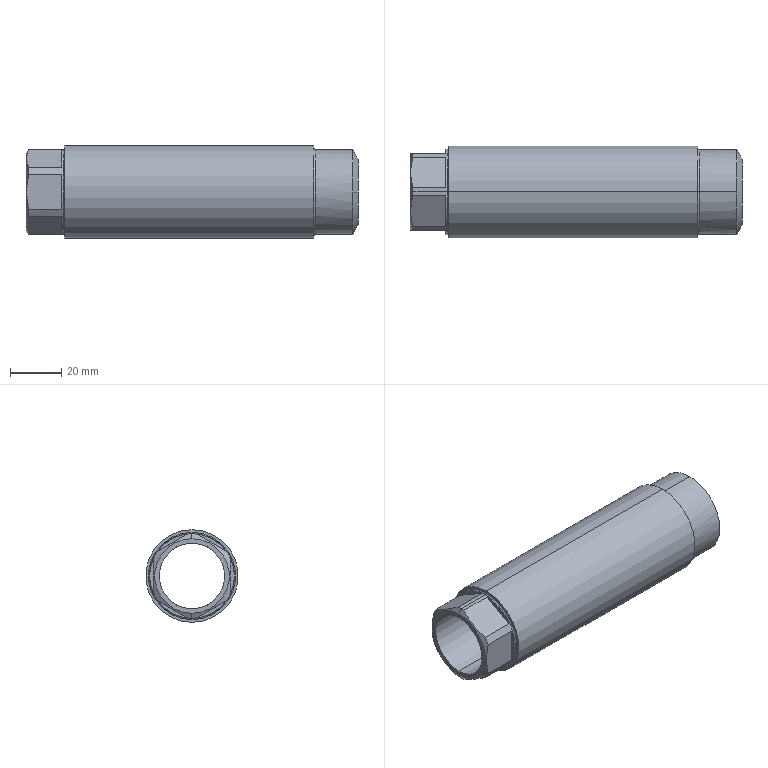Part | SolidWorks | features Cut 4, RevCut 2, Extrusion 1, Fillet 1 | 1 solid | 31 faces | box 129.156 x 36 x 36 mm | volume 58717 mm3 | plane 15 | cylinder 8 | torus 4 | cone 2 | sphere 2 | commonest cylinder face diameters 33 x4 25.5 x2 36 x2
STEP:
#1=CARTESIAN_POINT('',(0.,0.,-14.5));
#2=VERTEX_POINT('',#1);
#3=CARTESIAN_POINT('',(0.,0.,14.5));
#4=VERTEX_POINT('',#3);
#5=CARTESIAN_POINT('',(0.,0.,0.));
#6=DIRECTION('',(1.,0.,0.));
#7=DIRECTION('',(0.,0.,-1.));
#8=AXIS2_PLACEMENT_3D('',#5,#6,#7);
#9=CIRCLE('',#8,14.5);
#10=EDGE_CURVE('',#2,#4,#9,.T.);
#11=ORIENTED_EDGE('',*,*,#10,.T.);
#12=CARTESIAN_POINT('',(1.155,0.,16.5));
#13=VERTEX_POINT('',#12);
#14=CARTESIAN_POINT('',(5.774,0.,24.5));
#15=DIRECTION('',(0.5,0.,0.866));
#16=VECTOR('',#15,1000.);
#17=LINE('',#14,#16);
#18=EDGE_CURVE('',#4,#13,#17,.T.);
#19=ORIENTED_EDGE('',*,*,#18,.T.);
#20=CARTESIAN_POINT('',(1.155,1.547,16.427));
#21=VERTEX_POINT('',#20);
#22=CARTESIAN_POINT('',(1.155,0.,0.));
#23=DIRECTION('',(1.,0.,0.));
#24=DIRECTION('',(0.,0.,-1.));
#25=AXIS2_PLACEMENT_3D('',#22,#23,#24);
#26=CIRCLE('',#25,16.5);
#27=EDGE_CURVE('',#21,#13,#26,.T.);
#28=ORIENTED_EDGE('',*,*,#27,.F.);
#29=CARTESIAN_POINT('',(1.155,13.453,9.553));
#30=VERTEX_POINT('',#29);
#31=CARTESIAN_POINT('',(1.155,13.453,9.553));
#32=CARTESIAN_POINT('',(0.8829,12.474,10.119));
#33=CARTESIAN_POINT('',(0.6655,11.491,10.686));
#34=CARTESIAN_POINT('',(0.3687,9.515,11.827));
#35=CARTESIAN_POINT('',(0.2898,8.522,12.401));
#36=CARTESIAN_POINT('',(0.2881,7.022,13.266));
#37=CARTESIAN_POINT('',(0.3068,6.521,13.555));
#38=CARTESIAN_POINT('',(0.3828,5.516,14.136));
#39=CARTESIAN_POINT('',(0.44,5.013,14.426));
#40=CARTESIAN_POINT('',(0.6635,3.516,15.29));
#41=CARTESIAN_POINT('',(0.8823,2.528,15.861));
#42=CARTESIAN_POINT('',(1.155,1.547,16.427));
#43=B_SPLINE_CURVE_WITH_KNOTS('',3,(#31,#32,#33,#34,#35,#36,#37,#38,#39,#40,#41,#42),.UNSPECIFIED.,.F.,.F.,(4,2,2,2,2,4),(0.000000235,0.003449,0.006898,0.008623,0.01035,0.0138),.UNSPECIFIED.);
#44=EDGE_CURVE('',#30,#21,#43,.T.);
#45=ORIENTED_EDGE('',*,*,#44,.F.);
#46=CARTESIAN_POINT('',(1.155,15.,6.874));
#47=VERTEX_POINT('',#46);
#48=CARTESIAN_POINT('',(1.155,0.,0.));
#49=DIRECTION('',(1.,0.,0.));
#50=DIRECTION('',(0.,0.,-1.));
#51=AXIS2_PLACEMENT_3D('',#48,#49,#50);
#52=CIRCLE('',#51,16.5);
#53=EDGE_CURVE('',#47,#30,#52,.T.);
#54=ORIENTED_EDGE('',*,*,#53,.F.);
#55=CARTESIAN_POINT('',(1.155,15.,-6.874));
#56=VERTEX_POINT('',#55);
#57=CARTESIAN_POINT('',(1.155,15.,-6.874));
#58=CARTESIAN_POINT('',(0.8839,15.,-5.748));
#59=CARTESIAN_POINT('',(0.6635,15.,-4.599));
#60=CARTESIAN_POINT('',(0.3665,15.,-2.305));
#61=CARTESIAN_POINT('',(0.2888,15.,-1.155));
#62=CARTESIAN_POINT('',(0.2886,15.,1.15));
#63=CARTESIAN_POINT('',(0.3663,15.,2.307));
#64=CARTESIAN_POINT('',(0.6666,15.,4.619));
#65=CARTESIAN_POINT('',(0.8853,15.,5.754));
#66=CARTESIAN_POINT('',(1.155,15.,6.874));
#67=B_SPLINE_CURVE_WITH_KNOTS('',3,(#57,#58,#59,#60,#61,#62,#63,#64,#65,#66),.UNSPECIFIED.,.F.,.F.,(4,2,2,2,4),(0.01441,0.01786,0.02132,0.02477,0.02822),.UNSPECIFIED.);
#68=EDGE_CURVE('',#56,#47,#67,.T.);
#69=ORIENTED_EDGE('',*,*,#68,.F.);
#70=CARTESIAN_POINT('',(1.155,13.453,-9.553));
#71=VERTEX_POINT('',#70);
#72=CARTESIAN_POINT('',(1.155,0.,0.));
#73=DIRECTION('',(1.,0.,0.));
#74=DIRECTION('',(0.,0.,-1.));
#75=AXIS2_PLACEMENT_3D('',#72,#73,#74);
#76=CIRCLE('',#75,16.5);
#77=EDGE_CURVE('',#71,#56,#76,.T.);
#78=ORIENTED_EDGE('',*,*,#77,.F.);
#79=CARTESIAN_POINT('',(1.155,1.547,-16.427));
#80=VERTEX_POINT('',#79);
#81=CARTESIAN_POINT('',(1.155,1.547,-16.427));
#82=CARTESIAN_POINT('',(0.8829,2.526,-15.862));
#83=CARTESIAN_POINT('',(0.6655,3.509,-15.295));
#84=CARTESIAN_POINT('',(0.3687,5.485,-14.154));
#85=CARTESIAN_POINT('',(0.2898,6.478,-13.58));
#86=CARTESIAN_POINT('',(0.2881,7.978,-12.715));
#87=CARTESIAN_POINT('',(0.3068,8.479,-12.425));
#88=CARTESIAN_POINT('',(0.3828,9.484,-11.845));
#89=CARTESIAN_POINT('',(0.44,9.987,-11.555));
#90=CARTESIAN_POINT('',(0.6635,11.484,-10.69));
#91=CARTESIAN_POINT('',(0.8823,12.472,-10.12));
#92=CARTESIAN_POINT('',(1.155,13.453,-9.553));
#93=B_SPLINE_CURVE_WITH_KNOTS('',3,(#81,#82,#83,#84,#85,#86,#87,#88,#89,#90,#91,#92),.UNSPECIFIED.,.F.,.F.,(4,2,2,2,2,4),(0.000000235,0.003449,0.006898,0.008623,0.01035,0.0138),.UNSPECIFIED.);
#94=EDGE_CURVE('',#80,#71,#93,.T.);
#95=ORIENTED_EDGE('',*,*,#94,.F.);
#96=CARTESIAN_POINT('',(1.155,0.,-16.5));
#97=VERTEX_POINT('',#96);
#98=CARTESIAN_POINT('',(1.155,0.,0.));
#99=DIRECTION('',(1.,0.,0.));
#100=DIRECTION('',(0.,0.,-1.));
#101=AXIS2_PLACEMENT_3D('',#98,#99,#100);
#102=CIRCLE('',#101,16.5);
#103=EDGE_CURVE('',#97,#80,#102,.T.);
#104=ORIENTED_EDGE('',*,*,#103,.F.);
#105=CARTESIAN_POINT('',(5.774,0.,-24.5));
#106=DIRECTION('',(0.5,0.,-0.866));
#107=VECTOR('',#106,1000.);
#108=LINE('',#105,#107);
#109=EDGE_CURVE('',#2,#97,#108,.T.);
#110=ORIENTED_EDGE('',*,*,#109,.F.);
#111=EDGE_LOOP('',(#11,#19,#28,#45,#54,#69,#78,#95,#104,#110));
#112=FACE_OUTER_BOUND('',#111,.T.);
#113=CARTESIAN_POINT('',(5.774,0.,0.));
#114=DIRECTION('',(1.,0.,0.));
#115=DIRECTION('',(0.,0.,-1.));
#116=AXIS2_PLACEMENT_3D('',#113,#114,#115);
#117=CONICAL_SURFACE('',#116,24.5,1.047);
#118=ADVANCED_FACE('',(#112),#117,.T.);
#119=CARTESIAN_POINT('',(127.055,-16.5,0.));
#120=VERTEX_POINT('',#119);
#121=CARTESIAN_POINT('',(127.055,0.,16.5));
#122=VERTEX_POINT('',#121);
#123=CARTESIAN_POINT('',(127.055,0.,0.));
#124=DIRECTION('',(-1.,0.,0.));
#125=DIRECTION('',(0.,0.,1.));
#126=AXIS2_PLACEMENT_3D('',#123,#124,#125);
#127=CIRCLE('',#126,16.5);
#128=EDGE_CURVE('',#120,#122,#127,.T.);
#129=ORIENTED_EDGE('',*,*,#128,.F.);
#130=CARTESIAN_POINT('',(129.156,-12.75,0.));
#131=VERTEX_POINT('',#130);
#132=CARTESIAN_POINT('',(102.,0.,0.));
#133=DIRECTION('',(0.,0.,1.));
#134=DIRECTION('',(0.,-1.,0.));
#135=AXIS2_PLACEMENT_3D('',#132,#133,#134);
#136=CIRCLE('',#135,30.);
#137=EDGE_CURVE('',#120,#131,#136,.T.);
#138=ORIENTED_EDGE('',*,*,#137,.T.);
#139=CARTESIAN_POINT('',(129.156,0.,12.75));
#140=VERTEX_POINT('',#139);
#141=CARTESIAN_POINT('',(129.156,0.,0.));
#142=DIRECTION('',(-1.,0.,0.));
#143=DIRECTION('',(0.,0.,1.));
#144=AXIS2_PLACEMENT_3D('',#141,#142,#143);
#145=CIRCLE('',#144,12.75);
#146=EDGE_CURVE('',#131,#140,#145,.T.);
#147=ORIENTED_EDGE('',*,*,#146,.T.);
#148=CARTESIAN_POINT('',(129.156,12.75,0.));
#149=VERTEX_POINT('',#148);
#150=CARTESIAN_POINT('',(129.156,0.,0.));
#151=DIRECTION('',(-1.,0.,0.));
#152=DIRECTION('',(0.,0.,1.));
#153=AXIS2_PLACEMENT_3D('',#150,#151,#152);
#154=CIRCLE('',#153,12.75);
#155=EDGE_CURVE('',#140,#149,#154,.T.);
#156=ORIENTED_EDGE('',*,*,#155,.T.);
#157=CARTESIAN_POINT('',(127.055,16.5,0.));
#158=VERTEX_POINT('',#157);
#159=CARTESIAN_POINT('',(102.,0.,0.));
#160=DIRECTION('',(0.,0.,-1.));
#161=DIRECTION('',(-1.,0.,0.));
#162=AXIS2_PLACEMENT_3D('',#159,#160,#161);
#163=CIRCLE('',#162,30.);
#164=EDGE_CURVE('',#158,#149,#163,.T.);
#165=ORIENTED_EDGE('',*,*,#164,.F.);
#166=CARTESIAN_POINT('',(127.055,0.,0.));
#167=DIRECTION('',(-1.,0.,0.));
#168=DIRECTION('',(0.,0.,1.));
#169=AXIS2_PLACEMENT_3D('',#166,#167,#168);
#170=CIRCLE('',#169,16.5);
#171=EDGE_CURVE('',#122,#158,#170,.T.);
#172=ORIENTED_EDGE('',*,*,#171,.F.);
#173=EDGE_LOOP('',(#129,#138,#147,#156,#165,#172));
#174=FACE_OUTER_BOUND('',#173,.T.);
#175=CARTESIAN_POINT('',(102.,0.,0.));
#176=DIRECTION('',(0.,0.,1.));
#177=DIRECTION('',(0.,1.,0.));
#178=AXIS2_PLACEMENT_3D('',#175,#176,#177);
#179=SPHERICAL_SURFACE('',#178,30.);
#180=ADVANCED_FACE('',(#174),#179,.T.);
#181=CARTESIAN_POINT('',(112.5,0.,16.5));
#182=VERTEX_POINT('',#181);
#183=CARTESIAN_POINT('',(112.5,0.,-16.5));
#184=VERTEX_POINT('',#183);
#185=CARTESIAN_POINT('',(112.5,0.,0.));
#186=DIRECTION('',(1.,0.,0.));
#187=DIRECTION('',(0.,0.,-1.));
#188=AXIS2_PLACEMENT_3D('',#185,#186,#187);
#189=CIRCLE('',#188,16.5);
#190=EDGE_CURVE('',#182,#184,#189,.T.);
#191=ORIENTED_EDGE('',*,*,#190,.F.);
#192=CARTESIAN_POINT('',(112.,0.,17.));
#193=VERTEX_POINT('',#192);
#194=CARTESIAN_POINT('',(112.5,0.,17.));
#195=DIRECTION('',(0.,1.,0.));
#196=DIRECTION('',(0.,0.,1.));
#197=AXIS2_PLACEMENT_3D('',#194,#195,#196);
#198=CIRCLE('',#197,0.5);
#199=EDGE_CURVE('',#182,#193,#198,.T.);
#200=ORIENTED_EDGE('',*,*,#199,.T.);
#201=CARTESIAN_POINT('',(112.,0.,-17.));
#202=VERTEX_POINT('',#201);
#203=CARTESIAN_POINT('',(112.,0.,0.));
#204=DIRECTION('',(-1.,0.,0.));
#205=DIRECTION('',(0.,0.,-1.));
#206=AXIS2_PLACEMENT_3D('',#203,#204,#205);
#207=CIRCLE('',#206,17.);
#208=EDGE_CURVE('',#202,#193,#207,.T.);
#209=ORIENTED_EDGE('',*,*,#208,.F.);
#210=CARTESIAN_POINT('',(112.5,0.,-17.));
#211=DIRECTION('',(0.,-1.,0.));
#212=DIRECTION('',(0.,0.,-1.));
#213=AXIS2_PLACEMENT_3D('',#210,#211,#212);
#214=CIRCLE('',#213,0.5);
#215=EDGE_CURVE('',#184,#202,#214,.T.);
#216=ORIENTED_EDGE('',*,*,#215,.F.);
#217=EDGE_LOOP('',(#191,#200,#209,#216));
#218=FACE_OUTER_BOUND('',#217,.T.);
#219=CARTESIAN_POINT('',(112.5,0.,0.));
#220=DIRECTION('',(1.,0.,0.));
#221=DIRECTION('',(0.,0.,-1.));
#222=AXIS2_PLACEMENT_3D('',#219,#220,#221);
#223=TOROIDAL_SURFACE('',#222,17.,0.5);
#224=ADVANCED_FACE('',(#218),#223,.F.);
#225=CARTESIAN_POINT('',(14.5,0.,-16.5));
#226=VERTEX_POINT('',#225);
#227=CARTESIAN_POINT('',(14.5,0.,16.5));
#228=VERTEX_POINT('',#227);
#229=CARTESIAN_POINT('',(14.5,0.,0.));
#230=DIRECTION('',(-1.,0.,0.));
#231=DIRECTION('',(0.,0.,1.));
#232=AXIS2_PLACEMENT_3D('',#229,#230,#231);
#233=CIRCLE('',#232,16.5);
#234=EDGE_CURVE('',#226,#228,#233,.T.);
#235=ORIENTED_EDGE('',*,*,#234,.F.);
#236=CARTESIAN_POINT('',(15.,0.,-17.));
#237=VERTEX_POINT('',#236);
#238=CARTESIAN_POINT('',(14.5,0.,-17.));
#239=DIRECTION('',(0.,1.,0.));
#240=DIRECTION('',(0.,0.,1.));
#241=AXIS2_PLACEMENT_3D('',#238,#239,#240);
#242=CIRCLE('',#241,0.5);
#243=EDGE_CURVE('',#226,#237,#242,.T.);
#244=ORIENTED_EDGE('',*,*,#243,.T.);
#245=CARTESIAN_POINT('',(15.,0.,17.));
#246=VERTEX_POINT('',#245);
#247=CARTESIAN_POINT('',(15.,0.,0.));
#248=DIRECTION('',(1.,0.,0.));
#249=DIRECTION('',(0.,0.,1.));
#250=AXIS2_PLACEMENT_3D('',#247,#248,#249);
#251=CIRCLE('',#250,17.);
#252=EDGE_CURVE('',#246,#237,#251,.T.);
#253=ORIENTED_EDGE('',*,*,#252,.F.);
#254=CARTESIAN_POINT('',(14.5,0.,17.));
#255=DIRECTION('',(0.,-1.,0.));
#256=DIRECTION('',(0.,0.,-1.));
#257=AXIS2_PLACEMENT_3D('',#254,#255,#256);
#258=CIRCLE('',#257,0.5);
#259=EDGE_CURVE('',#228,#246,#258,.T.);
#260=ORIENTED_EDGE('',*,*,#259,.F.);
#261=EDGE_LOOP('',(#235,#244,#253,#260));
#262=FACE_OUTER_BOUND('',#261,.T.);
#263=CARTESIAN_POINT('',(14.5,0.,0.));
#264=DIRECTION('',(-1.,0.,0.));
#265=DIRECTION('',(0.,0.,1.));
#266=AXIS2_PLACEMENT_3D('',#263,#264,#265);
#267=TOROIDAL_SURFACE('',#266,17.,0.5);
#268=ADVANCED_FACE('',(#262),#267,.F.);
#269=CARTESIAN_POINT('',(112.,0.,-18.));
#270=VERTEX_POINT('',#269);
#271=CARTESIAN_POINT('',(112.,0.,18.));
#272=VERTEX_POINT('',#271);
#273=CARTESIAN_POINT('',(112.,0.,0.));
#274=DIRECTION('',(1.,0.,0.));
#275=DIRECTION('',(0.,0.,-1.));
#276=AXIS2_PLACEMENT_3D('',#273,#274,#275);
#277=CIRCLE('',#276,18.);
#278=EDGE_CURVE('',#270,#272,#277,.T.);
#279=ORIENTED_EDGE('',*,*,#278,.F.);
#280=CARTESIAN_POINT('',(15.,0.,-18.));
#281=VERTEX_POINT('',#280);
#282=CARTESIAN_POINT('',(132.,0.,-18.));
#283=DIRECTION('',(-1.,0.,0.));
#284=VECTOR('',#283,1000.);
#285=LINE('',#282,#284);
#286=EDGE_CURVE('',#270,#281,#285,.T.);
#287=ORIENTED_EDGE('',*,*,#286,.T.);
#288=CARTESIAN_POINT('',(15.,0.,18.));
#289=VERTEX_POINT('',#288);
#290=CARTESIAN_POINT('',(15.,0.,0.));
#291=DIRECTION('',(-1.,0.,0.));
#292=DIRECTION('',(0.,0.,1.));
#293=AXIS2_PLACEMENT_3D('',#290,#291,#292);
#294=CIRCLE('',#293,18.);
#295=EDGE_CURVE('',#289,#281,#294,.T.);
#296=ORIENTED_EDGE('',*,*,#295,.F.);
#297=CARTESIAN_POINT('',(132.,0.,18.));
#298=DIRECTION('',(-1.,0.,0.));
#299=VECTOR('',#298,1000.);
#300=LINE('',#297,#299);
#301=EDGE_CURVE('',#272,#289,#300,.T.);
#302=ORIENTED_EDGE('',*,*,#301,.F.);
#303=EDGE_LOOP('',(#279,#287,#296,#302));
#304=FACE_OUTER_BOUND('',#303,.T.);
#305=CARTESIAN_POINT('',(132.,0.,0.));
#306=DIRECTION('',(-1.,0.,0.));
#307=DIRECTION('',(0.,0.,1.));
#308=AXIS2_PLACEMENT_3D('',#305,#306,#307);
#309=CYLINDRICAL_SURFACE('',#308,18.);
#310=ADVANCED_FACE('',(#304),#309,.T.);
#311=CARTESIAN_POINT('',(112.5,0.,0.));
#312=DIRECTION('',(1.,0.,0.));
#313=DIRECTION('',(0.,0.,-1.));
#314=AXIS2_PLACEMENT_3D('',#311,#312,#313);
#315=CIRCLE('',#314,16.5);
#316=EDGE_CURVE('',#184,#182,#315,.T.);
#317=ORIENTED_EDGE('',*,*,#316,.T.);
#318=CARTESIAN_POINT('',(112.,0.,16.5));
#319=DIRECTION('',(1.,0.,0.));
#320=VECTOR('',#319,1000.);
#321=LINE('',#318,#320);
#322=EDGE_CURVE('',#182,#122,#321,.T.);
#323=ORIENTED_EDGE('',*,*,#322,.T.);
#324=ORIENTED_EDGE('',*,*,#171,.T.);
#325=CARTESIAN_POINT('',(127.055,0.,-16.5));
#326=VERTEX_POINT('',#325);
#327=CARTESIAN_POINT('',(127.055,0.,0.));
#328=DIRECTION('',(-1.,0.,0.));
#329=DIRECTION('',(0.,0.,1.));
#330=AXIS2_PLACEMENT_3D('',#327,#328,#329);
#331=CIRCLE('',#330,16.5);
#332=EDGE_CURVE('',#158,#326,#331,.T.);
#333=ORIENTED_EDGE('',*,*,#332,.T.);
#334=CARTESIAN_POINT('',(112.,0.,-16.5));
#335=DIRECTION('',(1.,0.,0.));
#336=VECTOR('',#335,1000.);
#337=LINE('',#334,#336);
#338=EDGE_CURVE('',#184,#326,#337,.T.);
#339=ORIENTED_EDGE('',*,*,#338,.F.);
#340=EDGE_LOOP('',(#317,#323,#324,#333,#339));
#341=FACE_OUTER_BOUND('',#340,.T.);
#342=CARTESIAN_POINT('',(112.,0.,0.));
#343=DIRECTION('',(1.,0.,0.));
#344=DIRECTION('',(0.,0.,-1.));
#345=AXIS2_PLACEMENT_3D('',#342,#343,#344);
#346=CYLINDRICAL_SURFACE('',#345,16.5);
#347=ADVANCED_FACE('',(#341),#346,.T.);
#348=CARTESIAN_POINT('',(129.156,0.,-12.75));
#349=VERTEX_POINT('',#348);
#350=CARTESIAN_POINT('',(129.156,0.,0.));
#351=DIRECTION('',(-1.,0.,0.));
#352=DIRECTION('',(0.,0.,1.));
#353=AXIS2_PLACEMENT_3D('',#350,#351,#352);
#354=CIRCLE('',#353,12.75);
#355=EDGE_CURVE('',#349,#131,#354,.T.);
#356=ORIENTED_EDGE('',*,*,#355,.F.);
#357=CARTESIAN_POINT('',(0.,0.,-12.75));
#358=VERTEX_POINT('',#357);
#359=CARTESIAN_POINT('',(132.,0.,-12.75));
#360=DIRECTION('',(-1.,0.,0.));
#361=VECTOR('',#360,1000.);
#362=LINE('',#359,#361);
#363=EDGE_CURVE('',#349,#358,#362,.T.);
#364=ORIENTED_EDGE('',*,*,#363,.T.);
#365=CARTESIAN_POINT('',(0.,0.,12.75));
#366=VERTEX_POINT('',#365);
#367=CARTESIAN_POINT('',(0.,0.,0.));
#368=DIRECTION('',(-1.,0.,0.));
#369=DIRECTION('',(0.,0.,1.));
#370=AXIS2_PLACEMENT_3D('',#367,#368,#369);
#371=CIRCLE('',#370,12.75);
#372=EDGE_CURVE('',#358,#366,#371,.T.);
#373=ORIENTED_EDGE('',*,*,#372,.T.);
#374=CARTESIAN_POINT('',(132.,0.,12.75));
#375=DIRECTION('',(-1.,0.,0.));
#376=VECTOR('',#375,1000.);
#377=LINE('',#374,#376);
#378=EDGE_CURVE('',#140,#366,#377,.T.);
#379=ORIENTED_EDGE('',*,*,#378,.F.);
#380=ORIENTED_EDGE('',*,*,#146,.F.);
#381=EDGE_LOOP('',(#356,#364,#373,#379,#380));
#382=FACE_OUTER_BOUND('',#381,.T.);
#383=CARTESIAN_POINT('',(132.,0.,0.));
#384=DIRECTION('',(-1.,0.,0.));
#385=DIRECTION('',(0.,0.,1.));
#386=AXIS2_PLACEMENT_3D('',#383,#384,#385);
#387=CYLINDRICAL_SURFACE('',#386,12.75);
#388=ADVANCED_FACE('',(#382),#387,.F.);
#389=CARTESIAN_POINT('',(14.5,0.,0.));
#390=DIRECTION('',(-1.,0.,0.));
#391=DIRECTION('',(0.,0.,1.));
#392=AXIS2_PLACEMENT_3D('',#389,#390,#391);
#393=CIRCLE('',#392,16.5);
#394=EDGE_CURVE('',#228,#226,#393,.T.);
#395=ORIENTED_EDGE('',*,*,#394,.T.);
#396=CARTESIAN_POINT('',(15.,0.,-16.5));
#397=DIRECTION('',(-1.,0.,0.));
#398=VECTOR('',#397,1000.);
#399=LINE('',#396,#398);
#400=EDGE_CURVE('',#226,#97,#399,.T.);
#401=ORIENTED_EDGE('',*,*,#400,.T.);
#402=ORIENTED_EDGE('',*,*,#103,.T.);
#403=CARTESIAN_POINT('',(14.,1.547,-16.427));
#404=VERTEX_POINT('',#403);
#405=CARTESIAN_POINT('',(15.,1.547,-16.427));
#406=DIRECTION('',(1.,0.,0.));
#407=VECTOR('',#406,1000.);
#408=LINE('',#405,#407);
#409=EDGE_CURVE('',#80,#404,#408,.T.);
#410=ORIENTED_EDGE('',*,*,#409,.T.);
#411=CARTESIAN_POINT('',(14.,13.453,-9.553));
#412=VERTEX_POINT('',#411);
#413=CARTESIAN_POINT('',(14.,0.,0.));
#414=DIRECTION('',(1.,0.,0.));
#415=DIRECTION('',(0.,0.,1.));
#416=AXIS2_PLACEMENT_3D('',#413,#414,#415);
#417=CIRCLE('',#416,16.5);
#418=EDGE_CURVE('',#404,#412,#417,.T.);
#419=ORIENTED_EDGE('',*,*,#418,.T.);
#420=CARTESIAN_POINT('',(15.,13.453,-9.553));
#421=DIRECTION('',(-1.,0.,0.));
#422=VECTOR('',#421,1000.);
#423=LINE('',#420,#422);
#424=EDGE_CURVE('',#412,#71,#423,.T.);
#425=ORIENTED_EDGE('',*,*,#424,.T.);
#426=ORIENTED_EDGE('',*,*,#77,.T.);
#427=CARTESIAN_POINT('',(14.,15.,-6.874));
#428=VERTEX_POINT('',#427);
#429=CARTESIAN_POINT('',(15.,15.,-6.874));
#430=DIRECTION('',(1.,0.,0.));
#431=VECTOR('',#430,1000.);
#432=LINE('',#429,#431);
#433=EDGE_CURVE('',#56,#428,#432,.T.);
#434=ORIENTED_EDGE('',*,*,#433,.T.);
#435=CARTESIAN_POINT('',(14.,15.,6.874));
#436=VERTEX_POINT('',#435);
#437=CARTESIAN_POINT('',(14.,0.,0.));
#438=DIRECTION('',(1.,0.,0.));
#439=DIRECTION('',(0.,0.,1.));
#440=AXIS2_PLACEMENT_3D('',#437,#438,#439);
#441=CIRCLE('',#440,16.5);
#442=EDGE_CURVE('',#428,#436,#441,.T.);
#443=ORIENTED_EDGE('',*,*,#442,.T.);
#444=CARTESIAN_POINT('',(15.,15.,6.874));
#445=DIRECTION('',(-1.,0.,0.));
#446=VECTOR('',#445,1000.);
#447=LINE('',#444,#446);
#448=EDGE_CURVE('',#436,#47,#447,.T.);
#449=ORIENTED_EDGE('',*,*,#448,.T.);
#450=ORIENTED_EDGE('',*,*,#53,.T.);
#451=CARTESIAN_POINT('',(14.,13.453,9.553));
#452=VERTEX_POINT('',#451);
#453=CARTESIAN_POINT('',(15.,13.453,9.553));
#454=DIRECTION('',(1.,0.,0.));
#455=VECTOR('',#454,1000.);
#456=LINE('',#453,#455);
#457=EDGE_CURVE('',#30,#452,#456,.T.);
#458=ORIENTED_EDGE('',*,*,#457,.T.);
#459=CARTESIAN_POINT('',(14.,1.547,16.427));
#460=VERTEX_POINT('',#459);
#461=CARTESIAN_POINT('',(14.,0.,0.));
#462=DIRECTION('',(1.,0.,0.));
#463=DIRECTION('',(0.,0.,1.));
#464=AXIS2_PLACEMENT_3D('',#461,#462,#463);
#465=CIRCLE('',#464,16.5);
#466=EDGE_CURVE('',#452,#460,#465,.T.);
#467=ORIENTED_EDGE('',*,*,#466,.T.);
#468=CARTESIAN_POINT('',(15.,1.547,16.427));
#469=DIRECTION('',(-1.,0.,0.));
#470=VECTOR('',#469,1000.);
#471=LINE('',#468,#470);
#472=EDGE_CURVE('',#460,#21,#471,.T.);
#473=ORIENTED_EDGE('',*,*,#472,.T.);
#474=ORIENTED_EDGE('',*,*,#27,.T.);
#475=CARTESIAN_POINT('',(15.,0.,16.5));
#476=DIRECTION('',(-1.,0.,0.));
#477=VECTOR('',#476,1000.);
#478=LINE('',#475,#477);
#479=EDGE_CURVE('',#228,#13,#478,.T.);
#480=ORIENTED_EDGE('',*,*,#479,.F.);
#481=EDGE_LOOP('',(#395,#401,#402,#410,#419,#425,#426,#434,#443,#449,#450,#458,#467,#473,#474,#480));
#482=FACE_OUTER_BOUND('',#481,.T.);
#483=CARTESIAN_POINT('',(15.,0.,0.));
#484=DIRECTION('',(-1.,0.,0.));
#485=DIRECTION('',(0.,0.,1.));
#486=AXIS2_PLACEMENT_3D('',#483,#484,#485);
#487=CYLINDRICAL_SURFACE('',#486,16.5);
#488=ADVANCED_FACE('',(#482),#487,.T.);
#489=CARTESIAN_POINT('',(0.,0.,0.));
#490=DIRECTION('',(-1.,0.,0.));
#491=DIRECTION('',(0.,0.,1.));
#492=AXIS2_PLACEMENT_3D('',#489,#490,#491);
#493=CIRCLE('',#492,12.75);
#494=EDGE_CURVE('',#366,#358,#493,.T.);
#495=ORIENTED_EDGE('',*,*,#494,.F.);
#496=ORIENTED_EDGE('',*,*,#372,.F.);
#497=EDGE_LOOP('',(#495,#496));
#498=FACE_BOUND('',#497,.T.);
#499=ORIENTED_EDGE('',*,*,#10,.F.);
#500=CARTESIAN_POINT('',(0.,0.,0.));
#501=DIRECTION('',(1.,0.,0.));
#502=DIRECTION('',(0.,0.,-1.));
#503=AXIS2_PLACEMENT_3D('',#500,#501,#502);
#504=CIRCLE('',#503,14.5);
#505=EDGE_CURVE('',#4,#2,#504,.T.);
#506=ORIENTED_EDGE('',*,*,#505,.F.);
#507=EDGE_LOOP('',(#499,#506));
#508=FACE_OUTER_BOUND('',#507,.T.);
#509=CARTESIAN_POINT('',(0.,0.,0.));
#510=DIRECTION('',(1.,0.,0.));
#511=DIRECTION('',(0.,0.,-1.));
#512=AXIS2_PLACEMENT_3D('',#509,#510,#511);
#513=PLANE('',#512);
#514=ADVANCED_FACE('',(#498,#508),#513,.F.);
#515=ORIENTED_EDGE('',*,*,#400,.F.);
#516=ORIENTED_EDGE('',*,*,#234,.T.);
#517=ORIENTED_EDGE('',*,*,#479,.T.);
#518=CARTESIAN_POINT('',(1.155,-1.547,16.427));
#519=VERTEX_POINT('',#518);
#520=CARTESIAN_POINT('',(1.155,0.,0.));
#521=DIRECTION('',(1.,0.,0.));
#522=DIRECTION('',(0.,0.,-1.));
#523=AXIS2_PLACEMENT_3D('',#520,#521,#522);
#524=CIRCLE('',#523,16.5);
#525=EDGE_CURVE('',#13,#519,#524,.T.);
#526=ORIENTED_EDGE('',*,*,#525,.T.);
#527=CARTESIAN_POINT('',(14.,-1.547,16.427));
#528=VERTEX_POINT('',#527);
#529=CARTESIAN_POINT('',(15.,-1.547,16.427));
#530=DIRECTION('',(1.,0.,0.));
#531=VECTOR('',#530,1000.);
#532=LINE('',#529,#531);
#533=EDGE_CURVE('',#519,#528,#532,.T.);
#534=ORIENTED_EDGE('',*,*,#533,.T.);
#535=CARTESIAN_POINT('',(14.,-13.453,9.553));
#536=VERTEX_POINT('',#535);
#537=CARTESIAN_POINT('',(14.,0.,0.));
#538=DIRECTION('',(1.,0.,0.));
#539=DIRECTION('',(0.,0.,1.));
#540=AXIS2_PLACEMENT_3D('',#537,#538,#539);
#541=CIRCLE('',#540,16.5);
#542=EDGE_CURVE('',#528,#536,#541,.T.);
#543=ORIENTED_EDGE('',*,*,#542,.T.);
#544=CARTESIAN_POINT('',(1.155,-13.453,9.553));
#545=VERTEX_POINT('',#544);
#546=CARTESIAN_POINT('',(15.,-13.453,9.553));
#547=DIRECTION('',(-1.,0.,0.));
#548=VECTOR('',#547,1000.);
#549=LINE('',#546,#548);
#550=EDGE_CURVE('',#536,#545,#549,.T.);
#551=ORIENTED_EDGE('',*,*,#550,.T.);
#552=CARTESIAN_POINT('',(1.155,-15.,6.874));
#553=VERTEX_POINT('',#552);
#554=CARTESIAN_POINT('',(1.155,0.,0.));
#555=DIRECTION('',(1.,0.,0.));
#556=DIRECTION('',(0.,0.,-1.));
#557=AXIS2_PLACEMENT_3D('',#554,#555,#556);
#558=CIRCLE('',#557,16.5);
#559=EDGE_CURVE('',#545,#553,#558,.T.);
#560=ORIENTED_EDGE('',*,*,#559,.T.);
#561=CARTESIAN_POINT('',(14.,-15.,6.874));
#562=VERTEX_POINT('',#561);
#563=CARTESIAN_POINT('',(15.,-15.,6.874));
#564=DIRECTION('',(1.,0.,0.));
#565=VECTOR('',#564,1000.);
#566=LINE('',#563,#565);
#567=EDGE_CURVE('',#553,#562,#566,.T.);
#568=ORIENTED_EDGE('',*,*,#567,.T.);
#569=CARTESIAN_POINT('',(14.,-15.,-6.874));
#570=VERTEX_POINT('',#569);
#571=CARTESIAN_POINT('',(14.,0.,0.));
#572=DIRECTION('',(1.,0.,0.));
#573=DIRECTION('',(0.,0.,1.));
#574=AXIS2_PLACEMENT_3D('',#571,#572,#573);
#575=CIRCLE('',#574,16.5);
#576=EDGE_CURVE('',#562,#570,#575,.T.);
#577=ORIENTED_EDGE('',*,*,#576,.T.);
#578=CARTESIAN_POINT('',(1.155,-15.,-6.874));
#579=VERTEX_POINT('',#578);
#580=CARTESIAN_POINT('',(15.,-15.,-6.874));
#581=DIRECTION('',(-1.,0.,0.));
#582=VECTOR('',#581,1000.);
#583=LINE('',#580,#582);
#584=EDGE_CURVE('',#570,#579,#583,.T.);
#585=ORIENTED_EDGE('',*,*,#584,.T.);
#586=CARTESIAN_POINT('',(1.155,-13.453,-9.553));
#587=VERTEX_POINT('',#586);
#588=CARTESIAN_POINT('',(1.155,0.,0.));
#589=DIRECTION('',(1.,0.,0.));
#590=DIRECTION('',(0.,0.,-1.));
#591=AXIS2_PLACEMENT_3D('',#588,#589,#590);
#592=CIRCLE('',#591,16.5);
#593=EDGE_CURVE('',#579,#587,#592,.T.);
#594=ORIENTED_EDGE('',*,*,#593,.T.);
#595=CARTESIAN_POINT('',(14.,-13.453,-9.553));
#596=VERTEX_POINT('',#595);
#597=CARTESIAN_POINT('',(15.,-13.453,-9.553));
#598=DIRECTION('',(1.,0.,0.));
#599=VECTOR('',#598,1000.);
#600=LINE('',#597,#599);
#601=EDGE_CURVE('',#587,#596,#600,.T.);
#602=ORIENTED_EDGE('',*,*,#601,.T.);
#603=CARTESIAN_POINT('',(14.,-1.547,-16.427));
#604=VERTEX_POINT('',#603);
#605=CARTESIAN_POINT('',(14.,0.,0.));
#606=DIRECTION('',(1.,0.,0.));
#607=DIRECTION('',(0.,0.,1.));
#608=AXIS2_PLACEMENT_3D('',#605,#606,#607);
#609=CIRCLE('',#608,16.5);
#610=EDGE_CURVE('',#596,#604,#609,.T.);
#611=ORIENTED_EDGE('',*,*,#610,.T.);
#612=CARTESIAN_POINT('',(1.155,-1.547,-16.427));
#613=VERTEX_POINT('',#612);
#614=CARTESIAN_POINT('',(15.,-1.547,-16.427));
#615=DIRECTION('',(-1.,0.,0.));
#616=VECTOR('',#615,1000.);
#617=LINE('',#614,#616);
#618=EDGE_CURVE('',#604,#613,#617,.T.);
#619=ORIENTED_EDGE('',*,*,#618,.T.);
#620=CARTESIAN_POINT('',(1.155,0.,0.));
#621=DIRECTION('',(1.,0.,0.));
#622=DIRECTION('',(0.,0.,-1.));
#623=AXIS2_PLACEMENT_3D('',#620,#621,#622);
#624=CIRCLE('',#623,16.5);
#625=EDGE_CURVE('',#613,#97,#624,.T.);
#626=ORIENTED_EDGE('',*,*,#625,.T.);
#627=EDGE_LOOP('',(#515,#516,#517,#526,#534,#543,#551,#560,#568,#577,#585,#594,#602,#611,#619,#626));
#628=FACE_OUTER_BOUND('',#627,.T.);
#629=CARTESIAN_POINT('',(15.,0.,0.));
#630=DIRECTION('',(-1.,0.,0.));
#631=DIRECTION('',(0.,0.,1.));
#632=AXIS2_PLACEMENT_3D('',#629,#630,#631);
#633=CYLINDRICAL_SURFACE('',#632,16.5);
#634=ADVANCED_FACE('',(#628),#633,.T.);
#635=ORIENTED_EDGE('',*,*,#567,.F.);
#636=CARTESIAN_POINT('',(1.155,-15.,6.874));
#637=CARTESIAN_POINT('',(0.8853,-15.,5.754));
#638=CARTESIAN_POINT('',(0.6666,-15.,4.619));
#639=CARTESIAN_POINT('',(0.3663,-15.,2.307));
#640=CARTESIAN_POINT('',(0.2886,-15.,1.15));
#641=CARTESIAN_POINT('',(0.2888,-15.,-1.155));
#642=CARTESIAN_POINT('',(0.3665,-15.,-2.305));
#643=CARTESIAN_POINT('',(0.6635,-15.,-4.599));
#644=CARTESIAN_POINT('',(0.8839,-15.,-5.748));
#645=CARTESIAN_POINT('',(1.155,-15.,-6.874));
#646=B_SPLINE_CURVE_WITH_KNOTS('',3,(#636,#637,#638,#639,#640,#641,#642,#643,#644,#645),.UNSPECIFIED.,.F.,.F.,(4,2,2,2,4),(0.01016,0.01361,0.01705,0.0205,0.02395),.UNSPECIFIED.);
#647=EDGE_CURVE('',#553,#579,#646,.T.);
#648=ORIENTED_EDGE('',*,*,#647,.T.);
#649=ORIENTED_EDGE('',*,*,#584,.F.);
#650=CARTESIAN_POINT('',(14.,-15.,-8.66));
#651=DIRECTION('',(0.,0.,1.));
#652=VECTOR('',#651,1000.);
#653=LINE('',#650,#652);
#654=EDGE_CURVE('',#570,#562,#653,.T.);
#655=ORIENTED_EDGE('',*,*,#654,.T.);
#656=EDGE_LOOP('',(#635,#648,#649,#655));
#657=FACE_OUTER_BOUND('',#656,.T.);
#658=CARTESIAN_POINT('',(14.,-15.,-8.66));
#659=DIRECTION('',(0.,-1.,0.));
#660=DIRECTION('',(0.,0.,-1.));
#661=AXIS2_PLACEMENT_3D('',#658,#659,#660);
#662=PLANE('',#661);
#663=ADVANCED_FACE('',(#657),#662,.T.);
#664=ORIENTED_EDGE('',*,*,#533,.F.);
#665=CARTESIAN_POINT('',(1.155,-1.547,16.427));
#666=CARTESIAN_POINT('',(0.8829,-2.526,15.862));
#667=CARTESIAN_POINT('',(0.6655,-3.509,15.295));
#668=CARTESIAN_POINT('',(0.3687,-5.485,14.154));
#669=CARTESIAN_POINT('',(0.2898,-6.478,13.58));
#670=CARTESIAN_POINT('',(0.2881,-7.978,12.715));
#671=CARTESIAN_POINT('',(0.3068,-8.479,12.425));
#672=CARTESIAN_POINT('',(0.3828,-9.484,11.845));
#673=CARTESIAN_POINT('',(0.44,-9.987,11.555));
#674=CARTESIAN_POINT('',(0.6635,-11.484,10.69));
#675=CARTESIAN_POINT('',(0.8823,-12.472,10.12));
#676=CARTESIAN_POINT('',(1.155,-13.453,9.553));
#677=B_SPLINE_CURVE_WITH_KNOTS('',3,(#665,#666,#667,#668,#669,#670,#671,#672,#673,#674,#675,#676),.UNSPECIFIED.,.F.,.F.,(4,2,2,2,2,4),(0.000000235,0.003449,0.006898,0.008623,0.01035,0.0138),.UNSPECIFIED.);
#678=EDGE_CURVE('',#519,#545,#677,.T.);
#679=ORIENTED_EDGE('',*,*,#678,.T.);
#680=ORIENTED_EDGE('',*,*,#550,.F.);
#681=CARTESIAN_POINT('',(14.,-15.,8.66));
#682=DIRECTION('',(0.,0.866,0.5));
#683=VECTOR('',#682,1000.);
#684=LINE('',#681,#683);
#685=EDGE_CURVE('',#536,#528,#684,.T.);
#686=ORIENTED_EDGE('',*,*,#685,.T.);
#687=EDGE_LOOP('',(#664,#679,#680,#686));
#688=FACE_OUTER_BOUND('',#687,.T.);
#689=CARTESIAN_POINT('',(14.,-15.,8.66));
#690=DIRECTION('',(0.,-0.5,0.866));
#691=DIRECTION('',(0.,-0.866,-0.5));
#692=AXIS2_PLACEMENT_3D('',#689,#690,#691);
#693=PLANE('',#692);
#694=ADVANCED_FACE('',(#688),#693,.T.);
#695=ORIENTED_EDGE('',*,*,#457,.F.);
#696=ORIENTED_EDGE('',*,*,#44,.T.);
#697=ORIENTED_EDGE('',*,*,#472,.F.);
#698=CARTESIAN_POINT('',(14.,0.,17.321));
#699=DIRECTION('',(0.,0.866,-0.5));
#700=VECTOR('',#699,1000.);
#701=LINE('',#698,#700);
#702=EDGE_CURVE('',#460,#452,#701,.T.);
#703=ORIENTED_EDGE('',*,*,#702,.T.);
#704=EDGE_LOOP('',(#695,#696,#697,#703));
#705=FACE_OUTER_BOUND('',#704,.T.);
#706=CARTESIAN_POINT('',(14.,0.,17.321));
#707=DIRECTION('',(0.,0.5,0.866));
#708=DIRECTION('',(0.,-0.866,0.5));
#709=AXIS2_PLACEMENT_3D('',#706,#707,#708);
#710=PLANE('',#709);
#711=ADVANCED_FACE('',(#705),#710,.T.);
#712=ORIENTED_EDGE('',*,*,#433,.F.);
#713=ORIENTED_EDGE('',*,*,#68,.T.);
#714=ORIENTED_EDGE('',*,*,#448,.F.);
#715=CARTESIAN_POINT('',(14.,15.,8.66));
#716=DIRECTION('',(0.,0.,-1.));
#717=VECTOR('',#716,1000.);
#718=LINE('',#715,#717);
#719=EDGE_CURVE('',#436,#428,#718,.T.);
#720=ORIENTED_EDGE('',*,*,#719,.T.);
#721=EDGE_LOOP('',(#712,#713,#714,#720));
#722=FACE_OUTER_BOUND('',#721,.T.);
#723=CARTESIAN_POINT('',(14.,15.,8.66));
#724=DIRECTION('',(0.,1.,0.));
#725=DIRECTION('',(0.,0.,1.));
#726=AXIS2_PLACEMENT_3D('',#723,#724,#725);
#727=PLANE('',#726);
#728=ADVANCED_FACE('',(#722),#727,.T.);
#729=ORIENTED_EDGE('',*,*,#409,.F.);
#730=ORIENTED_EDGE('',*,*,#94,.T.);
#731=ORIENTED_EDGE('',*,*,#424,.F.);
#732=CARTESIAN_POINT('',(14.,15.,-8.66));
#733=DIRECTION('',(0.,-0.866,-0.5));
#734=VECTOR('',#733,1000.);
#735=LINE('',#732,#734);
#736=EDGE_CURVE('',#412,#404,#735,.T.);
#737=ORIENTED_EDGE('',*,*,#736,.T.);
#738=EDGE_LOOP('',(#729,#730,#731,#737));
#739=FACE_OUTER_BOUND('',#738,.T.);
#740=CARTESIAN_POINT('',(14.,15.,-8.66));
#741=DIRECTION('',(0.,0.5,-0.866));
#742=DIRECTION('',(0.,0.866,0.5));
#743=AXIS2_PLACEMENT_3D('',#740,#741,#742);
#744=PLANE('',#743);
#745=ADVANCED_FACE('',(#739),#744,.T.);
#746=ORIENTED_EDGE('',*,*,#601,.F.);
#747=CARTESIAN_POINT('',(1.155,-13.453,-9.553));
#748=CARTESIAN_POINT('',(0.8829,-12.474,-10.119));
#749=CARTESIAN_POINT('',(0.6655,-11.491,-10.686));
#750=CARTESIAN_POINT('',(0.3687,-9.515,-11.827));
#751=CARTESIAN_POINT('',(0.2898,-8.522,-12.401));
#752=CARTESIAN_POINT('',(0.2881,-7.022,-13.266));
#753=CARTESIAN_POINT('',(0.3068,-6.521,-13.555));
#754=CARTESIAN_POINT('',(0.3828,-5.516,-14.136));
#755=CARTESIAN_POINT('',(0.44,-5.013,-14.426));
#756=CARTESIAN_POINT('',(0.6635,-3.516,-15.29));
#757=CARTESIAN_POINT('',(0.8823,-2.528,-15.861));
#758=CARTESIAN_POINT('',(1.155,-1.547,-16.427));
#759=B_SPLINE_CURVE_WITH_KNOTS('',3,(#747,#748,#749,#750,#751,#752,#753,#754,#755,#756,#757,#758),.UNSPECIFIED.,.F.,.F.,(4,2,2,2,2,4),(0.000000235,0.003449,0.006898,0.008623,0.01035,0.0138),.UNSPECIFIED.);
#760=EDGE_CURVE('',#587,#613,#759,.T.);
#761=ORIENTED_EDGE('',*,*,#760,.T.);
#762=ORIENTED_EDGE('',*,*,#618,.F.);
#763=CARTESIAN_POINT('',(14.,0.,-17.321));
#764=DIRECTION('',(0.,-0.866,0.5));
#765=VECTOR('',#764,1000.);
#766=LINE('',#763,#765);
#767=EDGE_CURVE('',#604,#596,#766,.T.);
#768=ORIENTED_EDGE('',*,*,#767,.T.);
#769=EDGE_LOOP('',(#746,#761,#762,#768));
#770=FACE_OUTER_BOUND('',#769,.T.);
#771=CARTESIAN_POINT('',(14.,0.,-17.321));
#772=DIRECTION('',(0.,-0.5,-0.866));
#773=DIRECTION('',(0.,0.866,-0.5));
#774=AXIS2_PLACEMENT_3D('',#771,#772,#773);
#775=PLANE('',#774);
#776=ADVANCED_FACE('',(#770),#775,.T.);
#777=ORIENTED_EDGE('',*,*,#363,.F.);
#778=CARTESIAN_POINT('',(129.156,0.,0.));
#779=DIRECTION('',(-1.,0.,0.));
#780=DIRECTION('',(0.,0.,1.));
#781=AXIS2_PLACEMENT_3D('',#778,#779,#780);
#782=CIRCLE('',#781,12.75);
#783=EDGE_CURVE('',#149,#349,#782,.T.);
#784=ORIENTED_EDGE('',*,*,#783,.F.);
#785=ORIENTED_EDGE('',*,*,#155,.F.);
#786=ORIENTED_EDGE('',*,*,#378,.T.);
#787=ORIENTED_EDGE('',*,*,#494,.T.);
#788=EDGE_LOOP('',(#777,#784,#785,#786,#787));
#789=FACE_OUTER_BOUND('',#788,.T.);
#790=CARTESIAN_POINT('',(132.,0.,0.));
#791=DIRECTION('',(-1.,0.,0.));
#792=DIRECTION('',(0.,0.,1.));
#793=AXIS2_PLACEMENT_3D('',#790,#791,#792);
#794=CYLINDRICAL_SURFACE('',#793,12.75);
#795=ADVANCED_FACE('',(#789),#794,.F.);
#796=ORIENTED_EDGE('',*,*,#322,.F.);
#797=ORIENTED_EDGE('',*,*,#190,.T.);
#798=ORIENTED_EDGE('',*,*,#338,.T.);
#799=CARTESIAN_POINT('',(127.055,0.,0.));
#800=DIRECTION('',(-1.,0.,0.));
#801=DIRECTION('',(0.,0.,1.));
#802=AXIS2_PLACEMENT_3D('',#799,#800,#801);
#803=CIRCLE('',#802,16.5);
#804=EDGE_CURVE('',#326,#120,#803,.T.);
#805=ORIENTED_EDGE('',*,*,#804,.T.);
#806=ORIENTED_EDGE('',*,*,#128,.T.);
#807=EDGE_LOOP('',(#796,#797,#798,#805,#806));
#808=FACE_OUTER_BOUND('',#807,.T.);
#809=CARTESIAN_POINT('',(112.,0.,0.));
#810=DIRECTION('',(1.,0.,0.));
#811=DIRECTION('',(0.,0.,-1.));
#812=AXIS2_PLACEMENT_3D('',#809,#810,#811);
#813=CYLINDRICAL_SURFACE('',#812,16.5);
#814=ADVANCED_FACE('',(#808),#813,.T.);
#815=ORIENTED_EDGE('',*,*,#286,.F.);
#816=CARTESIAN_POINT('',(112.,0.,0.));
#817=DIRECTION('',(1.,0.,0.));
#818=DIRECTION('',(0.,0.,-1.));
#819=AXIS2_PLACEMENT_3D('',#816,#817,#818);
#820=CIRCLE('',#819,18.);
#821=EDGE_CURVE('',#272,#270,#820,.T.);
#822=ORIENTED_EDGE('',*,*,#821,.F.);
#823=ORIENTED_EDGE('',*,*,#301,.T.);
#824=CARTESIAN_POINT('',(15.,0.,0.));
#825=DIRECTION('',(-1.,0.,0.));
#826=DIRECTION('',(0.,0.,1.));
#827=AXIS2_PLACEMENT_3D('',#824,#825,#826);
#828=CIRCLE('',#827,18.);
#829=EDGE_CURVE('',#281,#289,#828,.T.);
#830=ORIENTED_EDGE('',*,*,#829,.F.);
#831=EDGE_LOOP('',(#815,#822,#823,#830));
#832=FACE_OUTER_BOUND('',#831,.T.);
#833=CARTESIAN_POINT('',(132.,0.,0.));
#834=DIRECTION('',(-1.,0.,0.));
#835=DIRECTION('',(0.,0.,1.));
#836=AXIS2_PLACEMENT_3D('',#833,#834,#835);
#837=CYLINDRICAL_SURFACE('',#836,18.);
#838=ADVANCED_FACE('',(#832),#837,.T.);
#839=ORIENTED_EDGE('',*,*,#252,.T.);
#840=CARTESIAN_POINT('',(15.,0.,0.));
#841=DIRECTION('',(1.,0.,0.));
#842=DIRECTION('',(0.,0.,1.));
#843=AXIS2_PLACEMENT_3D('',#840,#841,#842);
#844=CIRCLE('',#843,17.);
#845=EDGE_CURVE('',#237,#246,#844,.T.);
#846=ORIENTED_EDGE('',*,*,#845,.T.);
#847=EDGE_LOOP('',(#839,#846));
#848=FACE_BOUND('',#847,.T.);
#849=ORIENTED_EDGE('',*,*,#295,.T.);
#850=ORIENTED_EDGE('',*,*,#829,.T.);
#851=EDGE_LOOP('',(#849,#850));
#852=FACE_OUTER_BOUND('',#851,.T.);
#853=CARTESIAN_POINT('',(15.,0.,0.));
#854=DIRECTION('',(-1.,0.,0.));
#855=DIRECTION('',(0.,0.,1.));
#856=AXIS2_PLACEMENT_3D('',#853,#854,#855);
#857=PLANE('',#856);
#858=ADVANCED_FACE('',(#848,#852),#857,.T.);
#859=ORIENTED_EDGE('',*,*,#208,.T.);
#860=CARTESIAN_POINT('',(112.,0.,0.));
#861=DIRECTION('',(-1.,0.,0.));
#862=DIRECTION('',(0.,0.,-1.));
#863=AXIS2_PLACEMENT_3D('',#860,#861,#862);
#864=CIRCLE('',#863,17.);
#865=EDGE_CURVE('',#193,#202,#864,.T.);
#866=ORIENTED_EDGE('',*,*,#865,.T.);
#867=EDGE_LOOP('',(#859,#866));
#868=FACE_BOUND('',#867,.T.);
#869=ORIENTED_EDGE('',*,*,#821,.T.);
#870=ORIENTED_EDGE('',*,*,#278,.T.);
#871=EDGE_LOOP('',(#869,#870));
#872=FACE_OUTER_BOUND('',#871,.T.);
#873=CARTESIAN_POINT('',(112.,0.,0.));
#874=DIRECTION('',(1.,0.,0.));
#875=DIRECTION('',(0.,0.,-1.));
#876=AXIS2_PLACEMENT_3D('',#873,#874,#875);
#877=PLANE('',#876);
#878=ADVANCED_FACE('',(#868,#872),#877,.T.);
#879=ORIENTED_EDGE('',*,*,#243,.F.);
#880=ORIENTED_EDGE('',*,*,#394,.F.);
#881=ORIENTED_EDGE('',*,*,#259,.T.);
#882=ORIENTED_EDGE('',*,*,#845,.F.);
#883=EDGE_LOOP('',(#879,#880,#881,#882));
#884=FACE_OUTER_BOUND('',#883,.T.);
#885=CARTESIAN_POINT('',(14.5,0.,0.));
#886=DIRECTION('',(-1.,0.,0.));
#887=DIRECTION('',(0.,0.,1.));
#888=AXIS2_PLACEMENT_3D('',#885,#886,#887);
#889=TOROIDAL_SURFACE('',#888,17.,0.5);
#890=ADVANCED_FACE('',(#884),#889,.F.);
#891=ORIENTED_EDGE('',*,*,#199,.F.);
#892=ORIENTED_EDGE('',*,*,#316,.F.);
#893=ORIENTED_EDGE('',*,*,#215,.T.);
#894=ORIENTED_EDGE('',*,*,#865,.F.);
#895=EDGE_LOOP('',(#891,#892,#893,#894));
#896=FACE_OUTER_BOUND('',#895,.T.);
#897=CARTESIAN_POINT('',(112.5,0.,0.));
#898=DIRECTION('',(1.,0.,0.));
#899=DIRECTION('',(0.,0.,-1.));
#900=AXIS2_PLACEMENT_3D('',#897,#898,#899);
#901=TOROIDAL_SURFACE('',#900,17.,0.5);
#902=ADVANCED_FACE('',(#896),#901,.F.);
#903=ORIENTED_EDGE('',*,*,#137,.F.);
#904=ORIENTED_EDGE('',*,*,#804,.F.);
#905=ORIENTED_EDGE('',*,*,#332,.F.);
#906=ORIENTED_EDGE('',*,*,#164,.T.);
#907=ORIENTED_EDGE('',*,*,#783,.T.);
#908=ORIENTED_EDGE('',*,*,#355,.T.);
#909=EDGE_LOOP('',(#903,#904,#905,#906,#907,#908));
#910=FACE_OUTER_BOUND('',#909,.T.);
#911=CARTESIAN_POINT('',(102.,0.,0.));
#912=DIRECTION('',(0.,0.,1.));
#913=DIRECTION('',(0.,1.,0.));
#914=AXIS2_PLACEMENT_3D('',#911,#912,#913);
#915=SPHERICAL_SURFACE('',#914,30.);
#916=ADVANCED_FACE('',(#910),#915,.T.);
#917=ORIENTED_EDGE('',*,*,#654,.F.);
#918=ORIENTED_EDGE('',*,*,#576,.F.);
#919=EDGE_LOOP('',(#917,#918));
#920=FACE_OUTER_BOUND('',#919,.T.);
#921=CARTESIAN_POINT('',(14.,0.,0.));
#922=DIRECTION('',(-1.,0.,0.));
#923=DIRECTION('',(0.,0.,1.));
#924=AXIS2_PLACEMENT_3D('',#921,#922,#923);
#925=PLANE('',#924);
#926=ADVANCED_FACE('',(#920),#925,.T.);
#927=ORIENTED_EDGE('',*,*,#685,.F.);
#928=ORIENTED_EDGE('',*,*,#542,.F.);
#929=EDGE_LOOP('',(#927,#928));
#930=FACE_OUTER_BOUND('',#929,.T.);
#931=CARTESIAN_POINT('',(14.,0.,0.));
#932=DIRECTION('',(-1.,0.,0.));
#933=DIRECTION('',(0.,0.,1.));
#934=AXIS2_PLACEMENT_3D('',#931,#932,#933);
#935=PLANE('',#934);
#936=ADVANCED_FACE('',(#930),#935,.T.);
#937=ORIENTED_EDGE('',*,*,#702,.F.);
#938=ORIENTED_EDGE('',*,*,#466,.F.);
#939=EDGE_LOOP('',(#937,#938));
#940=FACE_OUTER_BOUND('',#939,.T.);
#941=CARTESIAN_POINT('',(14.,0.,0.));
#942=DIRECTION('',(-1.,0.,0.));
#943=DIRECTION('',(0.,0.,1.));
#944=AXIS2_PLACEMENT_3D('',#941,#942,#943);
#945=PLANE('',#944);
#946=ADVANCED_FACE('',(#940),#945,.T.);
#947=ORIENTED_EDGE('',*,*,#719,.F.);
#948=ORIENTED_EDGE('',*,*,#442,.F.);
#949=EDGE_LOOP('',(#947,#948));
#950=FACE_OUTER_BOUND('',#949,.T.);
#951=CARTESIAN_POINT('',(14.,0.,0.));
#952=DIRECTION('',(-1.,0.,0.));
#953=DIRECTION('',(0.,0.,1.));
#954=AXIS2_PLACEMENT_3D('',#951,#952,#953);
#955=PLANE('',#954);
#956=ADVANCED_FACE('',(#950),#955,.T.);
#957=ORIENTED_EDGE('',*,*,#736,.F.);
#958=ORIENTED_EDGE('',*,*,#418,.F.);
#959=EDGE_LOOP('',(#957,#958));
#960=FACE_OUTER_BOUND('',#959,.T.);
#961=CARTESIAN_POINT('',(14.,0.,0.));
#962=DIRECTION('',(-1.,0.,0.));
#963=DIRECTION('',(0.,0.,1.));
#964=AXIS2_PLACEMENT_3D('',#961,#962,#963);
#965=PLANE('',#964);
#966=ADVANCED_FACE('',(#960),#965,.T.);
#967=ORIENTED_EDGE('',*,*,#767,.F.);
#968=ORIENTED_EDGE('',*,*,#610,.F.);
#969=EDGE_LOOP('',(#967,#968));
#970=FACE_OUTER_BOUND('',#969,.T.);
#971=CARTESIAN_POINT('',(14.,0.,0.));
#972=DIRECTION('',(-1.,0.,0.));
#973=DIRECTION('',(0.,0.,1.));
#974=AXIS2_PLACEMENT_3D('',#971,#972,#973);
#975=PLANE('',#974);
#976=ADVANCED_FACE('',(#970),#975,.T.);
#977=ORIENTED_EDGE('',*,*,#18,.F.);
#978=ORIENTED_EDGE('',*,*,#505,.T.);
#979=ORIENTED_EDGE('',*,*,#109,.T.);
#980=ORIENTED_EDGE('',*,*,#625,.F.);
#981=ORIENTED_EDGE('',*,*,#760,.F.);
#982=ORIENTED_EDGE('',*,*,#593,.F.);
#983=ORIENTED_EDGE('',*,*,#647,.F.);
#984=ORIENTED_EDGE('',*,*,#559,.F.);
#985=ORIENTED_EDGE('',*,*,#678,.F.);
#986=ORIENTED_EDGE('',*,*,#525,.F.);
#987=EDGE_LOOP('',(#977,#978,#979,#980,#981,#982,#983,#984,#985,#986));
#988=FACE_OUTER_BOUND('',#987,.T.);
#989=CARTESIAN_POINT('',(5.774,0.,0.));
#990=DIRECTION('',(1.,0.,0.));
#991=DIRECTION('',(0.,0.,-1.));
#992=AXIS2_PLACEMENT_3D('',#989,#990,#991);
#993=CONICAL_SURFACE('',#992,24.5,1.047);
#994=ADVANCED_FACE('',(#988),#993,.T.);
#995=CLOSED_SHELL('',(#118,#180,#224,#268,#310,#347,#388,#488,#514,#634,#663,#694,#711,#728,#745,#776,#795,#814,#838,#858,#878,#890,#902,#916,#926,#936,#946,#956,#966,#976,#994));
#996=MANIFOLD_SOLID_BREP('',#995);
#997=CARTESIAN_POINT('',(0.,0.,0.));
#998=DIRECTION('',(0.,0.,1.));
#999=DIRECTION('',(1.,0.,0.));
#1000=AXIS2_PLACEMENT_3D('',#997,#998,#999);
#1001=(LENGTH_UNIT()NAMED_UNIT(*)SI_UNIT(.MILLI.,.METRE.));
#1002=UNCERTAINTY_MEASURE_WITH_UNIT(LENGTH_MEASURE(0.00001),#1001,'','');
#1003=(NAMED_UNIT(*)PLANE_ANGLE_UNIT()SI_UNIT($,.RADIAN.));
#1004=(NAMED_UNIT(*)SI_UNIT($,.STERADIAN.)SOLID_ANGLE_UNIT());
#1005=(GEOMETRIC_REPRESENTATION_CONTEXT(3)GLOBAL_UNCERTAINTY_ASSIGNED_CONTEXT((#1002))GLOBAL_UNIT_ASSIGNED_CONTEXT((#1001,#1003,#1004))REPRESENTATION_CONTEXT('',''));
#1006=ADVANCED_BREP_SHAPE_REPRESENTATION('',(#996,#1000),#1005);